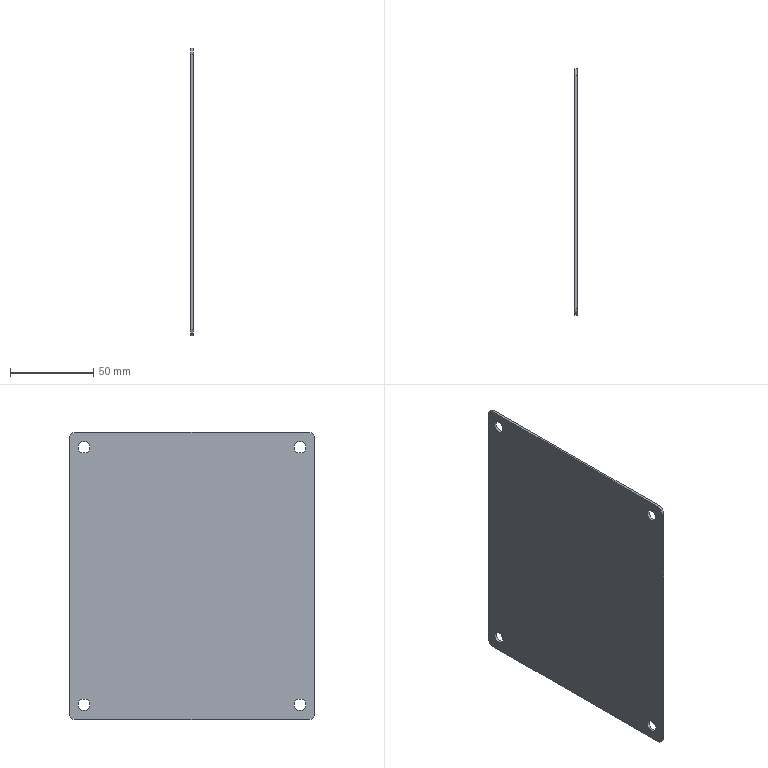Part | NX | features solid 2 | 1 solid | 18 faces | box 1.5 x 148 x 173 mm | volume 38154 mm3 | cylinder 12 | plane 6 | commonest cylinder face diameters 7 x8 8 x4
STEP:
#1=CARTESIAN_POINT('',(1098.5,-1223.5,-585.));
#2=VERTEX_POINT('',#1);
#3=CARTESIAN_POINT('',(1100.,-1223.5,-585.));
#4=VERTEX_POINT('',#3);
#5=CARTESIAN_POINT('',(872.326,-1223.5,-585.));
#6=DIRECTION('',(1.,0.,0.));
#7=VECTOR('',#6,1000.);
#8=LINE('',#5,#7);
#9=EDGE_CURVE('',#2,#4,#8,.T.);
#10=ORIENTED_EDGE('',*,*,#9,.F.);
#11=CARTESIAN_POINT('',(1098.5,-1216.5,-585.));
#12=VERTEX_POINT('',#11);
#13=CARTESIAN_POINT('',(1098.5,-1220.,-585.));
#14=DIRECTION('',(-1.,0.,0.));
#15=DIRECTION('',(0.,-1.,0.));
#16=AXIS2_PLACEMENT_3D('',#13,#14,#15);
#17=CIRCLE('',#16,3.5);
#18=EDGE_CURVE('',#2,#12,#17,.T.);
#19=ORIENTED_EDGE('',*,*,#18,.T.);
#20=CARTESIAN_POINT('',(1100.,-1216.5,-585.));
#21=VERTEX_POINT('',#20);
#22=CARTESIAN_POINT('',(872.326,-1216.5,-585.));
#23=DIRECTION('',(1.,0.,0.));
#24=VECTOR('',#23,1000.);
#25=LINE('',#22,#24);
#26=EDGE_CURVE('',#21,#12,#25,.F.);
#27=ORIENTED_EDGE('',*,*,#26,.F.);
#28=CARTESIAN_POINT('',(1100.,-1220.,-585.));
#29=DIRECTION('',(1.,0.,0.));
#30=DIRECTION('',(0.,1.,0.));
#31=AXIS2_PLACEMENT_3D('',#28,#29,#30);
#32=CIRCLE('',#31,3.5);
#33=EDGE_CURVE('',#21,#4,#32,.T.);
#34=ORIENTED_EDGE('',*,*,#33,.T.);
#35=EDGE_LOOP('',(#10,#19,#27,#34));
#36=FACE_BOUND('',#35,.T.);
#37=CARTESIAN_POINT('',(872.326,-1220.,-585.));
#38=DIRECTION('',(1.,0.,0.));
#39=DIRECTION('',(0.,1.,0.));
#40=AXIS2_PLACEMENT_3D('',#37,#38,#39);
#41=CYLINDRICAL_SURFACE('',#40,3.5);
#42=ADVANCED_FACE('',(#36),#41,.F.);
#43=CARTESIAN_POINT('',(1100.,-1093.5,-585.));
#44=VERTEX_POINT('',#43);
#45=CARTESIAN_POINT('',(1098.5,-1093.5,-585.));
#46=VERTEX_POINT('',#45);
#47=CARTESIAN_POINT('',(872.326,-1093.5,-585.));
#48=DIRECTION('',(1.,0.,0.));
#49=VECTOR('',#48,1000.);
#50=LINE('',#47,#49);
#51=EDGE_CURVE('',#44,#46,#50,.F.);
#52=ORIENTED_EDGE('',*,*,#51,.T.);
#53=CARTESIAN_POINT('',(1098.5,-1086.5,-585.));
#54=VERTEX_POINT('',#53);
#55=CARTESIAN_POINT('',(1098.5,-1090.,-585.));
#56=DIRECTION('',(-1.,0.,0.));
#57=DIRECTION('',(0.,-1.,0.));
#58=AXIS2_PLACEMENT_3D('',#55,#56,#57);
#59=CIRCLE('',#58,3.5);
#60=EDGE_CURVE('',#46,#54,#59,.T.);
#61=ORIENTED_EDGE('',*,*,#60,.T.);
#62=CARTESIAN_POINT('',(1100.,-1086.5,-585.));
#63=VERTEX_POINT('',#62);
#64=CARTESIAN_POINT('',(872.326,-1086.5,-585.));
#65=DIRECTION('',(1.,0.,0.));
#66=VECTOR('',#65,1000.);
#67=LINE('',#64,#66);
#68=EDGE_CURVE('',#54,#63,#67,.T.);
#69=ORIENTED_EDGE('',*,*,#68,.T.);
#70=CARTESIAN_POINT('',(1100.,-1090.,-585.));
#71=DIRECTION('',(1.,0.,0.));
#72=DIRECTION('',(0.,1.,0.));
#73=AXIS2_PLACEMENT_3D('',#70,#71,#72);
#74=CIRCLE('',#73,3.5);
#75=EDGE_CURVE('',#63,#44,#74,.T.);
#76=ORIENTED_EDGE('',*,*,#75,.T.);
#77=EDGE_LOOP('',(#52,#61,#69,#76));
#78=FACE_BOUND('',#77,.T.);
#79=CARTESIAN_POINT('',(872.326,-1090.,-585.));
#80=DIRECTION('',(1.,0.,0.));
#81=DIRECTION('',(0.,1.,0.));
#82=AXIS2_PLACEMENT_3D('',#79,#80,#81);
#83=CYLINDRICAL_SURFACE('',#82,3.5);
#84=ADVANCED_FACE('',(#78),#83,.F.);
#85=CARTESIAN_POINT('',(1098.5,-1093.5,-430.));
#86=VERTEX_POINT('',#85);
#87=CARTESIAN_POINT('',(1100.,-1093.5,-430.));
#88=VERTEX_POINT('',#87);
#89=CARTESIAN_POINT('',(872.326,-1093.5,-430.));
#90=DIRECTION('',(1.,0.,0.));
#91=VECTOR('',#90,1000.);
#92=LINE('',#89,#91);
#93=EDGE_CURVE('',#86,#88,#92,.T.);
#94=ORIENTED_EDGE('',*,*,#93,.F.);
#95=CARTESIAN_POINT('',(1098.5,-1086.5,-430.));
#96=VERTEX_POINT('',#95);
#97=CARTESIAN_POINT('',(1098.5,-1090.,-430.));
#98=DIRECTION('',(-1.,0.,0.));
#99=DIRECTION('',(0.,-1.,0.));
#100=AXIS2_PLACEMENT_3D('',#97,#98,#99);
#101=CIRCLE('',#100,3.5);
#102=EDGE_CURVE('',#86,#96,#101,.T.);
#103=ORIENTED_EDGE('',*,*,#102,.T.);
#104=CARTESIAN_POINT('',(1100.,-1086.5,-430.));
#105=VERTEX_POINT('',#104);
#106=CARTESIAN_POINT('',(872.326,-1086.5,-430.));
#107=DIRECTION('',(1.,0.,0.));
#108=VECTOR('',#107,1000.);
#109=LINE('',#106,#108);
#110=EDGE_CURVE('',#105,#96,#109,.F.);
#111=ORIENTED_EDGE('',*,*,#110,.F.);
#112=CARTESIAN_POINT('',(1100.,-1090.,-430.));
#113=DIRECTION('',(1.,0.,0.));
#114=DIRECTION('',(0.,1.,0.));
#115=AXIS2_PLACEMENT_3D('',#112,#113,#114);
#116=CIRCLE('',#115,3.5);
#117=EDGE_CURVE('',#105,#88,#116,.T.);
#118=ORIENTED_EDGE('',*,*,#117,.T.);
#119=EDGE_LOOP('',(#94,#103,#111,#118));
#120=FACE_BOUND('',#119,.T.);
#121=CARTESIAN_POINT('',(872.326,-1090.,-430.));
#122=DIRECTION('',(1.,0.,0.));
#123=DIRECTION('',(0.,1.,0.));
#124=AXIS2_PLACEMENT_3D('',#121,#122,#123);
#125=CYLINDRICAL_SURFACE('',#124,3.5);
#126=ADVANCED_FACE('',(#120),#125,.F.);
#127=CARTESIAN_POINT('',(1098.5,-1223.5,-430.));
#128=VERTEX_POINT('',#127);
#129=CARTESIAN_POINT('',(1100.,-1223.5,-430.));
#130=VERTEX_POINT('',#129);
#131=CARTESIAN_POINT('',(872.326,-1223.5,-430.));
#132=DIRECTION('',(1.,0.,0.));
#133=VECTOR('',#132,1000.);
#134=LINE('',#131,#133);
#135=EDGE_CURVE('',#128,#130,#134,.T.);
#136=ORIENTED_EDGE('',*,*,#135,.F.);
#137=CARTESIAN_POINT('',(1098.5,-1216.5,-430.));
#138=VERTEX_POINT('',#137);
#139=CARTESIAN_POINT('',(1098.5,-1220.,-430.));
#140=DIRECTION('',(-1.,0.,0.));
#141=DIRECTION('',(0.,-1.,0.));
#142=AXIS2_PLACEMENT_3D('',#139,#140,#141);
#143=CIRCLE('',#142,3.5);
#144=EDGE_CURVE('',#128,#138,#143,.T.);
#145=ORIENTED_EDGE('',*,*,#144,.T.);
#146=CARTESIAN_POINT('',(1100.,-1216.5,-430.));
#147=VERTEX_POINT('',#146);
#148=CARTESIAN_POINT('',(872.326,-1216.5,-430.));
#149=DIRECTION('',(1.,0.,0.));
#150=VECTOR('',#149,1000.);
#151=LINE('',#148,#150);
#152=EDGE_CURVE('',#147,#138,#151,.F.);
#153=ORIENTED_EDGE('',*,*,#152,.F.);
#154=CARTESIAN_POINT('',(1100.,-1220.,-430.));
#155=DIRECTION('',(1.,0.,0.));
#156=DIRECTION('',(0.,1.,0.));
#157=AXIS2_PLACEMENT_3D('',#154,#155,#156);
#158=CIRCLE('',#157,3.5);
#159=EDGE_CURVE('',#147,#130,#158,.T.);
#160=ORIENTED_EDGE('',*,*,#159,.T.);
#161=EDGE_LOOP('',(#136,#145,#153,#160));
#162=FACE_BOUND('',#161,.T.);
#163=CARTESIAN_POINT('',(872.326,-1220.,-430.));
#164=DIRECTION('',(1.,0.,0.));
#165=DIRECTION('',(0.,1.,0.));
#166=AXIS2_PLACEMENT_3D('',#163,#164,#165);
#167=CYLINDRICAL_SURFACE('',#166,3.5);
#168=ADVANCED_FACE('',(#162),#167,.F.);
#169=ORIENTED_EDGE('',*,*,#159,.F.);
#170=CARTESIAN_POINT('',(1100.,-1220.,-430.));
#171=DIRECTION('',(1.,0.,0.));
#172=DIRECTION('',(0.,1.,0.));
#173=AXIS2_PLACEMENT_3D('',#170,#171,#172);
#174=CIRCLE('',#173,3.5);
#175=EDGE_CURVE('',#130,#147,#174,.T.);
#176=ORIENTED_EDGE('',*,*,#175,.F.);
#177=EDGE_LOOP('',(#169,#176));
#178=FACE_BOUND('',#177,.T.);
#179=ORIENTED_EDGE('',*,*,#117,.F.);
#180=CARTESIAN_POINT('',(1100.,-1090.,-430.));
#181=DIRECTION('',(1.,0.,0.));
#182=DIRECTION('',(0.,1.,0.));
#183=AXIS2_PLACEMENT_3D('',#180,#181,#182);
#184=CIRCLE('',#183,3.5);
#185=EDGE_CURVE('',#88,#105,#184,.T.);
#186=ORIENTED_EDGE('',*,*,#185,.F.);
#187=EDGE_LOOP('',(#179,#186));
#188=FACE_BOUND('',#187,.T.);
#189=ORIENTED_EDGE('',*,*,#75,.F.);
#190=CARTESIAN_POINT('',(1100.,-1090.,-585.));
#191=DIRECTION('',(1.,0.,0.));
#192=DIRECTION('',(0.,1.,0.));
#193=AXIS2_PLACEMENT_3D('',#190,#191,#192);
#194=CIRCLE('',#193,3.5);
#195=EDGE_CURVE('',#44,#63,#194,.T.);
#196=ORIENTED_EDGE('',*,*,#195,.F.);
#197=EDGE_LOOP('',(#189,#196));
#198=FACE_BOUND('',#197,.T.);
#199=ORIENTED_EDGE('',*,*,#33,.F.);
#200=CARTESIAN_POINT('',(1100.,-1220.,-585.));
#201=DIRECTION('',(1.,0.,0.));
#202=DIRECTION('',(0.,1.,0.));
#203=AXIS2_PLACEMENT_3D('',#200,#201,#202);
#204=CIRCLE('',#203,3.5);
#205=EDGE_CURVE('',#4,#21,#204,.T.);
#206=ORIENTED_EDGE('',*,*,#205,.F.);
#207=EDGE_LOOP('',(#199,#206));
#208=FACE_BOUND('',#207,.T.);
#209=CARTESIAN_POINT('',(1100.,-1229.,-425.));
#210=VERTEX_POINT('',#209);
#211=CARTESIAN_POINT('',(1100.,-1225.,-421.));
#212=VERTEX_POINT('',#211);
#213=CARTESIAN_POINT('',(1100.,-1225.,-425.));
#214=DIRECTION('',(-1.,0.,0.));
#215=DIRECTION('',(0.,1.,0.));
#216=AXIS2_PLACEMENT_3D('',#213,#214,#215);
#217=CIRCLE('',#216,4.);
#218=EDGE_CURVE('',#210,#212,#217,.T.);
#219=ORIENTED_EDGE('',*,*,#218,.F.);
#220=CARTESIAN_POINT('',(1100.,-1229.,-590.));
#221=VERTEX_POINT('',#220);
#222=CARTESIAN_POINT('',(1100.,-1229.,-590.));
#223=DIRECTION('',(0.,0.,1.));
#224=VECTOR('',#223,1000.);
#225=LINE('',#222,#224);
#226=EDGE_CURVE('',#221,#210,#225,.T.);
#227=ORIENTED_EDGE('',*,*,#226,.F.);
#228=CARTESIAN_POINT('',(1100.,-1225.,-594.));
#229=VERTEX_POINT('',#228);
#230=CARTESIAN_POINT('',(1100.,-1225.,-590.));
#231=DIRECTION('',(-1.,0.,0.));
#232=DIRECTION('',(0.,1.,0.));
#233=AXIS2_PLACEMENT_3D('',#230,#231,#232);
#234=CIRCLE('',#233,4.);
#235=EDGE_CURVE('',#229,#221,#234,.T.);
#236=ORIENTED_EDGE('',*,*,#235,.F.);
#237=CARTESIAN_POINT('',(1100.,-1085.,-594.));
#238=VERTEX_POINT('',#237);
#239=CARTESIAN_POINT('',(1100.,-1085.,-594.));
#240=DIRECTION('',(0.,-1.,0.));
#241=VECTOR('',#240,1000.);
#242=LINE('',#239,#241);
#243=EDGE_CURVE('',#238,#229,#242,.T.);
#244=ORIENTED_EDGE('',*,*,#243,.F.);
#245=CARTESIAN_POINT('',(1100.,-1081.,-590.));
#246=VERTEX_POINT('',#245);
#247=CARTESIAN_POINT('',(1100.,-1085.,-590.));
#248=DIRECTION('',(-1.,0.,0.));
#249=DIRECTION('',(0.,1.,0.));
#250=AXIS2_PLACEMENT_3D('',#247,#248,#249);
#251=CIRCLE('',#250,4.);
#252=EDGE_CURVE('',#246,#238,#251,.T.);
#253=ORIENTED_EDGE('',*,*,#252,.F.);
#254=CARTESIAN_POINT('',(1100.,-1081.,-425.));
#255=VERTEX_POINT('',#254);
#256=CARTESIAN_POINT('',(1100.,-1081.,-425.));
#257=DIRECTION('',(0.,0.,-1.));
#258=VECTOR('',#257,1000.);
#259=LINE('',#256,#258);
#260=EDGE_CURVE('',#255,#246,#259,.T.);
#261=ORIENTED_EDGE('',*,*,#260,.F.);
#262=CARTESIAN_POINT('',(1100.,-1085.,-421.));
#263=VERTEX_POINT('',#262);
#264=CARTESIAN_POINT('',(1100.,-1085.,-425.));
#265=DIRECTION('',(-1.,0.,0.));
#266=DIRECTION('',(0.,-1.,0.));
#267=AXIS2_PLACEMENT_3D('',#264,#265,#266);
#268=CIRCLE('',#267,4.);
#269=EDGE_CURVE('',#263,#255,#268,.T.);
#270=ORIENTED_EDGE('',*,*,#269,.F.);
#271=CARTESIAN_POINT('',(1100.,-1225.,-421.));
#272=DIRECTION('',(0.,1.,0.));
#273=VECTOR('',#272,1000.);
#274=LINE('',#271,#273);
#275=EDGE_CURVE('',#212,#263,#274,.T.);
#276=ORIENTED_EDGE('',*,*,#275,.F.);
#277=EDGE_LOOP('',(#219,#227,#236,#244,#253,#261,#270,#276));
#278=FACE_BOUND('',#277,.T.);
#279=CARTESIAN_POINT('',(1100.,-1225.,-425.));
#280=DIRECTION('',(-1.,0.,0.));
#281=DIRECTION('',(0.,0.,1.));
#282=AXIS2_PLACEMENT_3D('',#279,#280,#281);
#283=PLANE('',#282);
#284=ADVANCED_FACE('',(#178,#188,#198,#208,#278),#283,.F.);
#285=CARTESIAN_POINT('',(1098.5,-1220.,-430.));
#286=DIRECTION('',(-1.,0.,0.));
#287=DIRECTION('',(0.,-1.,0.));
#288=AXIS2_PLACEMENT_3D('',#285,#286,#287);
#289=CIRCLE('',#288,3.5);
#290=EDGE_CURVE('',#138,#128,#289,.T.);
#291=ORIENTED_EDGE('',*,*,#290,.F.);
#292=ORIENTED_EDGE('',*,*,#144,.F.);
#293=EDGE_LOOP('',(#291,#292));
#294=FACE_BOUND('',#293,.T.);
#295=CARTESIAN_POINT('',(1098.5,-1090.,-430.));
#296=DIRECTION('',(-1.,0.,0.));
#297=DIRECTION('',(0.,-1.,0.));
#298=AXIS2_PLACEMENT_3D('',#295,#296,#297);
#299=CIRCLE('',#298,3.5);
#300=EDGE_CURVE('',#96,#86,#299,.T.);
#301=ORIENTED_EDGE('',*,*,#300,.F.);
#302=ORIENTED_EDGE('',*,*,#102,.F.);
#303=EDGE_LOOP('',(#301,#302));
#304=FACE_BOUND('',#303,.T.);
#305=CARTESIAN_POINT('',(1098.5,-1090.,-585.));
#306=DIRECTION('',(-1.,0.,0.));
#307=DIRECTION('',(0.,-1.,0.));
#308=AXIS2_PLACEMENT_3D('',#305,#306,#307);
#309=CIRCLE('',#308,3.5);
#310=EDGE_CURVE('',#54,#46,#309,.T.);
#311=ORIENTED_EDGE('',*,*,#310,.F.);
#312=ORIENTED_EDGE('',*,*,#60,.F.);
#313=EDGE_LOOP('',(#311,#312));
#314=FACE_BOUND('',#313,.T.);
#315=CARTESIAN_POINT('',(1098.5,-1220.,-585.));
#316=DIRECTION('',(-1.,0.,0.));
#317=DIRECTION('',(0.,-1.,0.));
#318=AXIS2_PLACEMENT_3D('',#315,#316,#317);
#319=CIRCLE('',#318,3.5);
#320=EDGE_CURVE('',#12,#2,#319,.T.);
#321=ORIENTED_EDGE('',*,*,#320,.F.);
#322=ORIENTED_EDGE('',*,*,#18,.F.);
#323=EDGE_LOOP('',(#321,#322));
#324=FACE_BOUND('',#323,.T.);
#325=CARTESIAN_POINT('',(1098.5,-1229.,-425.));
#326=VERTEX_POINT('',#325);
#327=CARTESIAN_POINT('',(1098.5,-1225.,-421.));
#328=VERTEX_POINT('',#327);
#329=CARTESIAN_POINT('',(1098.5,-1225.,-425.));
#330=DIRECTION('',(-1.,0.,0.));
#331=DIRECTION('',(0.,1.,0.));
#332=AXIS2_PLACEMENT_3D('',#329,#330,#331);
#333=CIRCLE('',#332,4.);
#334=EDGE_CURVE('',#326,#328,#333,.T.);
#335=ORIENTED_EDGE('',*,*,#334,.T.);
#336=CARTESIAN_POINT('',(1098.5,-1085.,-421.));
#337=VERTEX_POINT('',#336);
#338=CARTESIAN_POINT('',(1098.5,-1225.,-421.));
#339=DIRECTION('',(0.,1.,0.));
#340=VECTOR('',#339,1000.);
#341=LINE('',#338,#340);
#342=EDGE_CURVE('',#328,#337,#341,.T.);
#343=ORIENTED_EDGE('',*,*,#342,.T.);
#344=CARTESIAN_POINT('',(1098.5,-1081.,-425.));
#345=VERTEX_POINT('',#344);
#346=CARTESIAN_POINT('',(1098.5,-1085.,-425.));
#347=DIRECTION('',(-1.,0.,0.));
#348=DIRECTION('',(0.,-1.,0.));
#349=AXIS2_PLACEMENT_3D('',#346,#347,#348);
#350=CIRCLE('',#349,4.);
#351=EDGE_CURVE('',#337,#345,#350,.T.);
#352=ORIENTED_EDGE('',*,*,#351,.T.);
#353=CARTESIAN_POINT('',(1098.5,-1081.,-590.));
#354=VERTEX_POINT('',#353);
#355=CARTESIAN_POINT('',(1098.5,-1081.,-425.));
#356=DIRECTION('',(0.,0.,-1.));
#357=VECTOR('',#356,1000.);
#358=LINE('',#355,#357);
#359=EDGE_CURVE('',#345,#354,#358,.T.);
#360=ORIENTED_EDGE('',*,*,#359,.T.);
#361=CARTESIAN_POINT('',(1098.5,-1085.,-594.));
#362=VERTEX_POINT('',#361);
#363=CARTESIAN_POINT('',(1098.5,-1085.,-590.));
#364=DIRECTION('',(-1.,0.,0.));
#365=DIRECTION('',(0.,1.,0.));
#366=AXIS2_PLACEMENT_3D('',#363,#364,#365);
#367=CIRCLE('',#366,4.);
#368=EDGE_CURVE('',#354,#362,#367,.T.);
#369=ORIENTED_EDGE('',*,*,#368,.T.);
#370=CARTESIAN_POINT('',(1098.5,-1225.,-594.));
#371=VERTEX_POINT('',#370);
#372=CARTESIAN_POINT('',(1098.5,-1085.,-594.));
#373=DIRECTION('',(0.,-1.,0.));
#374=VECTOR('',#373,1000.);
#375=LINE('',#372,#374);
#376=EDGE_CURVE('',#362,#371,#375,.T.);
#377=ORIENTED_EDGE('',*,*,#376,.T.);
#378=CARTESIAN_POINT('',(1098.5,-1229.,-590.));
#379=VERTEX_POINT('',#378);
#380=CARTESIAN_POINT('',(1098.5,-1225.,-590.));
#381=DIRECTION('',(-1.,0.,0.));
#382=DIRECTION('',(0.,1.,0.));
#383=AXIS2_PLACEMENT_3D('',#380,#381,#382);
#384=CIRCLE('',#383,4.);
#385=EDGE_CURVE('',#371,#379,#384,.T.);
#386=ORIENTED_EDGE('',*,*,#385,.T.);
#387=CARTESIAN_POINT('',(1098.5,-1229.,-590.));
#388=DIRECTION('',(0.,0.,1.));
#389=VECTOR('',#388,1000.);
#390=LINE('',#387,#389);
#391=EDGE_CURVE('',#379,#326,#390,.T.);
#392=ORIENTED_EDGE('',*,*,#391,.T.);
#393=EDGE_LOOP('',(#335,#343,#352,#360,#369,#377,#386,#392));
#394=FACE_BOUND('',#393,.T.);
#395=CARTESIAN_POINT('',(1098.5,-1225.,-425.));
#396=DIRECTION('',(-1.,0.,0.));
#397=DIRECTION('',(0.,0.,1.));
#398=AXIS2_PLACEMENT_3D('',#395,#396,#397);
#399=PLANE('',#398);
#400=ADVANCED_FACE('',(#294,#304,#314,#324,#394),#399,.T.);
#401=ORIENTED_EDGE('',*,*,#226,.T.);
#402=CARTESIAN_POINT('',(1098.5,-1229.,-425.));
#403=DIRECTION('',(1.,0.,0.));
#404=VECTOR('',#403,1000.);
#405=LINE('',#402,#404);
#406=EDGE_CURVE('',#326,#210,#405,.T.);
#407=ORIENTED_EDGE('',*,*,#406,.F.);
#408=ORIENTED_EDGE('',*,*,#391,.F.);
#409=CARTESIAN_POINT('',(1098.5,-1229.,-590.));
#410=DIRECTION('',(1.,0.,0.));
#411=VECTOR('',#410,1000.);
#412=LINE('',#409,#411);
#413=EDGE_CURVE('',#379,#221,#412,.T.);
#414=ORIENTED_EDGE('',*,*,#413,.T.);
#415=EDGE_LOOP('',(#401,#407,#408,#414));
#416=FACE_BOUND('',#415,.T.);
#417=CARTESIAN_POINT('',(1098.5,-1229.,-590.));
#418=DIRECTION('',(0.,1.,0.));
#419=DIRECTION('',(0.,0.,-1.));
#420=AXIS2_PLACEMENT_3D('',#417,#418,#419);
#421=PLANE('',#420);
#422=ADVANCED_FACE('',(#416),#421,.F.);
#423=ORIENTED_EDGE('',*,*,#235,.T.);
#424=ORIENTED_EDGE('',*,*,#413,.F.);
#425=ORIENTED_EDGE('',*,*,#385,.F.);
#426=CARTESIAN_POINT('',(1098.5,-1225.,-594.));
#427=DIRECTION('',(1.,0.,0.));
#428=VECTOR('',#427,1000.);
#429=LINE('',#426,#428);
#430=EDGE_CURVE('',#371,#229,#429,.T.);
#431=ORIENTED_EDGE('',*,*,#430,.T.);
#432=EDGE_LOOP('',(#423,#424,#425,#431));
#433=FACE_BOUND('',#432,.T.);
#434=CARTESIAN_POINT('',(1098.5,-1225.,-590.));
#435=DIRECTION('',(1.,0.,0.));
#436=DIRECTION('',(0.,0.,-1.));
#437=AXIS2_PLACEMENT_3D('',#434,#435,#436);
#438=CYLINDRICAL_SURFACE('',#437,4.);
#439=ADVANCED_FACE('',(#433),#438,.T.);
#440=ORIENTED_EDGE('',*,*,#243,.T.);
#441=ORIENTED_EDGE('',*,*,#430,.F.);
#442=ORIENTED_EDGE('',*,*,#376,.F.);
#443=CARTESIAN_POINT('',(1098.5,-1085.,-594.));
#444=DIRECTION('',(1.,0.,0.));
#445=VECTOR('',#444,1000.);
#446=LINE('',#443,#445);
#447=EDGE_CURVE('',#362,#238,#446,.T.);
#448=ORIENTED_EDGE('',*,*,#447,.T.);
#449=EDGE_LOOP('',(#440,#441,#442,#448));
#450=FACE_BOUND('',#449,.T.);
#451=CARTESIAN_POINT('',(1098.5,-1085.,-594.));
#452=DIRECTION('',(0.,0.,1.));
#453=DIRECTION('',(1.,0.,0.));
#454=AXIS2_PLACEMENT_3D('',#451,#452,#453);
#455=PLANE('',#454);
#456=ADVANCED_FACE('',(#450),#455,.F.);
#457=ORIENTED_EDGE('',*,*,#252,.T.);
#458=ORIENTED_EDGE('',*,*,#447,.F.);
#459=ORIENTED_EDGE('',*,*,#368,.F.);
#460=CARTESIAN_POINT('',(1098.5,-1081.,-590.));
#461=DIRECTION('',(1.,0.,0.));
#462=VECTOR('',#461,1000.);
#463=LINE('',#460,#462);
#464=EDGE_CURVE('',#354,#246,#463,.T.);
#465=ORIENTED_EDGE('',*,*,#464,.T.);
#466=EDGE_LOOP('',(#457,#458,#459,#465));
#467=FACE_BOUND('',#466,.T.);
#468=CARTESIAN_POINT('',(1098.5,-1085.,-590.));
#469=DIRECTION('',(1.,0.,0.));
#470=DIRECTION('',(0.,0.,-1.));
#471=AXIS2_PLACEMENT_3D('',#468,#469,#470);
#472=CYLINDRICAL_SURFACE('',#471,4.);
#473=ADVANCED_FACE('',(#467),#472,.T.);
#474=ORIENTED_EDGE('',*,*,#260,.T.);
#475=ORIENTED_EDGE('',*,*,#464,.F.);
#476=ORIENTED_EDGE('',*,*,#359,.F.);
#477=CARTESIAN_POINT('',(1098.5,-1081.,-425.));
#478=DIRECTION('',(1.,0.,0.));
#479=VECTOR('',#478,1000.);
#480=LINE('',#477,#479);
#481=EDGE_CURVE('',#345,#255,#480,.T.);
#482=ORIENTED_EDGE('',*,*,#481,.T.);
#483=EDGE_LOOP('',(#474,#475,#476,#482));
#484=FACE_BOUND('',#483,.T.);
#485=CARTESIAN_POINT('',(1098.5,-1081.,-425.));
#486=DIRECTION('',(0.,-1.,0.));
#487=DIRECTION('',(-1.,0.,0.));
#488=AXIS2_PLACEMENT_3D('',#485,#486,#487);
#489=PLANE('',#488);
#490=ADVANCED_FACE('',(#484),#489,.F.);
#491=ORIENTED_EDGE('',*,*,#269,.T.);
#492=ORIENTED_EDGE('',*,*,#481,.F.);
#493=ORIENTED_EDGE('',*,*,#351,.F.);
#494=CARTESIAN_POINT('',(1098.5,-1085.,-421.));
#495=DIRECTION('',(1.,0.,0.));
#496=VECTOR('',#495,1000.);
#497=LINE('',#494,#496);
#498=EDGE_CURVE('',#337,#263,#497,.T.);
#499=ORIENTED_EDGE('',*,*,#498,.T.);
#500=EDGE_LOOP('',(#491,#492,#493,#499));
#501=FACE_BOUND('',#500,.T.);
#502=CARTESIAN_POINT('',(1098.5,-1085.,-425.));
#503=DIRECTION('',(1.,0.,0.));
#504=DIRECTION('',(0.,0.,-1.));
#505=AXIS2_PLACEMENT_3D('',#502,#503,#504);
#506=CYLINDRICAL_SURFACE('',#505,4.);
#507=ADVANCED_FACE('',(#501),#506,.T.);
#508=ORIENTED_EDGE('',*,*,#275,.T.);
#509=ORIENTED_EDGE('',*,*,#498,.F.);
#510=ORIENTED_EDGE('',*,*,#342,.F.);
#511=CARTESIAN_POINT('',(1098.5,-1225.,-421.));
#512=DIRECTION('',(1.,0.,0.));
#513=VECTOR('',#512,1000.);
#514=LINE('',#511,#513);
#515=EDGE_CURVE('',#328,#212,#514,.T.);
#516=ORIENTED_EDGE('',*,*,#515,.T.);
#517=EDGE_LOOP('',(#508,#509,#510,#516));
#518=FACE_BOUND('',#517,.T.);
#519=CARTESIAN_POINT('',(1098.5,-1225.,-421.));
#520=DIRECTION('',(0.,0.,-1.));
#521=DIRECTION('',(0.,-1.,0.));
#522=AXIS2_PLACEMENT_3D('',#519,#520,#521);
#523=PLANE('',#522);
#524=ADVANCED_FACE('',(#518),#523,.F.);
#525=ORIENTED_EDGE('',*,*,#218,.T.);
#526=ORIENTED_EDGE('',*,*,#515,.F.);
#527=ORIENTED_EDGE('',*,*,#334,.F.);
#528=ORIENTED_EDGE('',*,*,#406,.T.);
#529=EDGE_LOOP('',(#525,#526,#527,#528));
#530=FACE_BOUND('',#529,.T.);
#531=CARTESIAN_POINT('',(1098.5,-1225.,-425.));
#532=DIRECTION('',(1.,0.,0.));
#533=DIRECTION('',(0.,0.,-1.));
#534=AXIS2_PLACEMENT_3D('',#531,#532,#533);
#535=CYLINDRICAL_SURFACE('',#534,4.);
#536=ADVANCED_FACE('',(#530),#535,.T.);
#537=ORIENTED_EDGE('',*,*,#290,.T.);
#538=ORIENTED_EDGE('',*,*,#135,.T.);
#539=ORIENTED_EDGE('',*,*,#175,.T.);
#540=ORIENTED_EDGE('',*,*,#152,.T.);
#541=EDGE_LOOP('',(#537,#538,#539,#540));
#542=FACE_BOUND('',#541,.T.);
#543=CARTESIAN_POINT('',(872.326,-1220.,-430.));
#544=DIRECTION('',(1.,0.,0.));
#545=DIRECTION('',(0.,1.,0.));
#546=AXIS2_PLACEMENT_3D('',#543,#544,#545);
#547=CYLINDRICAL_SURFACE('',#546,3.5);
#548=ADVANCED_FACE('',(#542),#547,.F.);
#549=ORIENTED_EDGE('',*,*,#300,.T.);
#550=ORIENTED_EDGE('',*,*,#93,.T.);
#551=ORIENTED_EDGE('',*,*,#185,.T.);
#552=ORIENTED_EDGE('',*,*,#110,.T.);
#553=EDGE_LOOP('',(#549,#550,#551,#552));
#554=FACE_BOUND('',#553,.T.);
#555=CARTESIAN_POINT('',(872.326,-1090.,-430.));
#556=DIRECTION('',(1.,0.,0.));
#557=DIRECTION('',(0.,1.,0.));
#558=AXIS2_PLACEMENT_3D('',#555,#556,#557);
#559=CYLINDRICAL_SURFACE('',#558,3.5);
#560=ADVANCED_FACE('',(#554),#559,.F.);
#561=ORIENTED_EDGE('',*,*,#310,.T.);
#562=ORIENTED_EDGE('',*,*,#51,.F.);
#563=ORIENTED_EDGE('',*,*,#195,.T.);
#564=ORIENTED_EDGE('',*,*,#68,.F.);
#565=EDGE_LOOP('',(#561,#562,#563,#564));
#566=FACE_BOUND('',#565,.T.);
#567=CARTESIAN_POINT('',(872.326,-1090.,-585.));
#568=DIRECTION('',(1.,0.,0.));
#569=DIRECTION('',(0.,1.,0.));
#570=AXIS2_PLACEMENT_3D('',#567,#568,#569);
#571=CYLINDRICAL_SURFACE('',#570,3.5);
#572=ADVANCED_FACE('',(#566),#571,.F.);
#573=ORIENTED_EDGE('',*,*,#320,.T.);
#574=ORIENTED_EDGE('',*,*,#9,.T.);
#575=ORIENTED_EDGE('',*,*,#205,.T.);
#576=ORIENTED_EDGE('',*,*,#26,.T.);
#577=EDGE_LOOP('',(#573,#574,#575,#576));
#578=FACE_BOUND('',#577,.T.);
#579=CARTESIAN_POINT('',(872.326,-1220.,-585.));
#580=DIRECTION('',(1.,0.,0.));
#581=DIRECTION('',(0.,1.,0.));
#582=AXIS2_PLACEMENT_3D('',#579,#580,#581);
#583=CYLINDRICAL_SURFACE('',#582,3.5);
#584=ADVANCED_FACE('',(#578),#583,.F.);
#585=CLOSED_SHELL('',(#42,#84,#126,#168,#284,#400,#422,#439,#456,#473,#490,#507,#524,#536,#548,#560,#572,#584));
#586=MANIFOLD_SOLID_BREP('',#585);
#587=(LENGTH_UNIT()NAMED_UNIT(*)SI_UNIT(.MILLI.,.METRE.));
#588=UNCERTAINTY_MEASURE_WITH_UNIT(LENGTH_MEASURE(0.00001),#587,'','');
#589=(NAMED_UNIT(*)PLANE_ANGLE_UNIT()SI_UNIT($,.RADIAN.));
#590=(NAMED_UNIT(*)SI_UNIT($,.STERADIAN.)SOLID_ANGLE_UNIT());
#591=(GEOMETRIC_REPRESENTATION_CONTEXT(3)GLOBAL_UNCERTAINTY_ASSIGNED_CONTEXT((#588))GLOBAL_UNIT_ASSIGNED_CONTEXT((#587,#589,#590))REPRESENTATION_CONTEXT('',''));
#592=ADVANCED_BREP_SHAPE_REPRESENTATION('',(#586),#591);